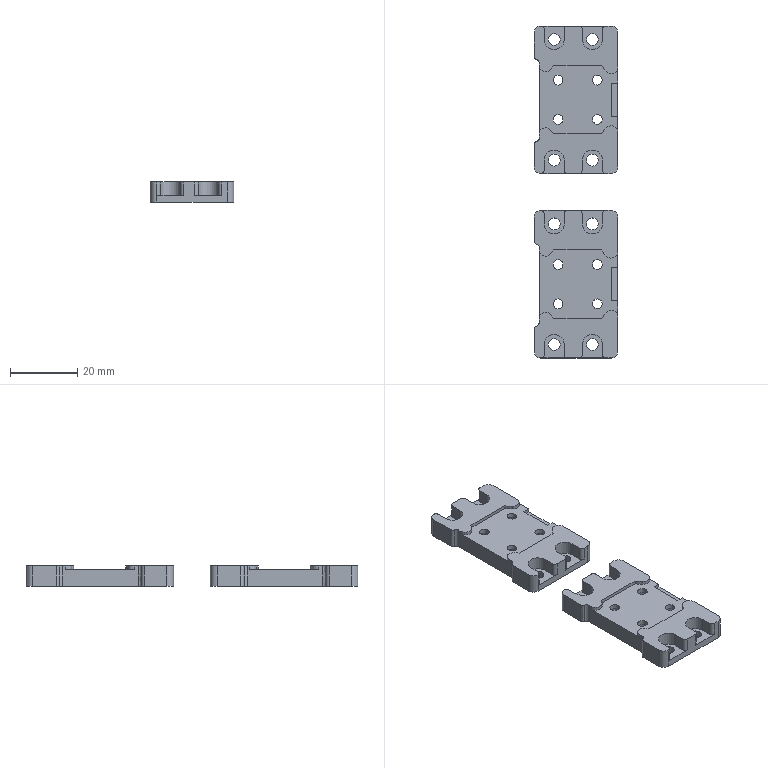Part | 2 solids | 152 faces | box 25 x 99 x 6 mm | volume 9568 mm3 | cylinder 72 | plane 64 | spline 8 | cone 8 | commonest cylinder face diameters 2 x20 4 x12 2.9 x8 3.5 x8 5.5 x8 6 x8